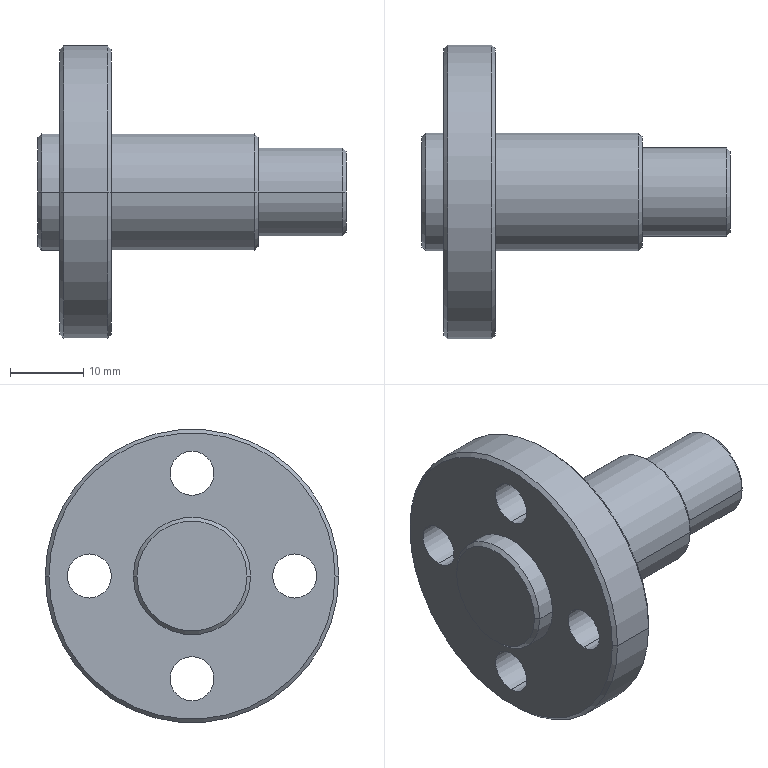Part | STEP file | PN_0036 Shaft_Default | 1 solid | 31 faces | box 42 x 40 x 40 mm | volume 13938 mm3 | cylinder 16 | cone 10 | plane 5 | commonest cylinder face diameters 6 x8 16 x4 12 x2 40 x2